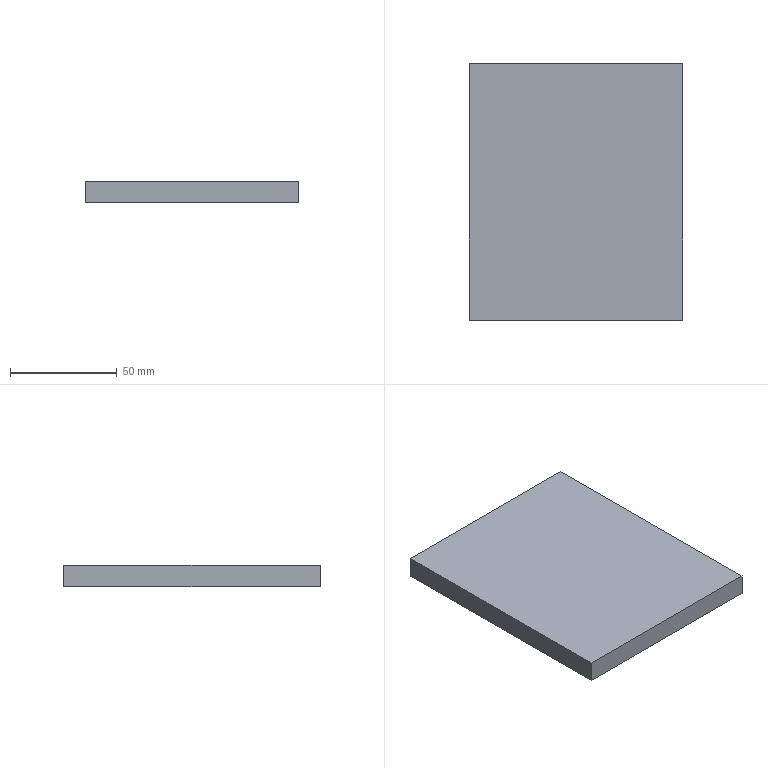Part | SolidWorks | features ICE 3, Extrusion 1 | 1 solid | 6 faces | box 100 x 120 x 10 mm | volume 120000 mm3 | plane 6
STEP:
#1=CARTESIAN_POINT('',(50.,100.,10.));
#2=VERTEX_POINT('',#1);
#3=CARTESIAN_POINT('',(50.,100.,0.));
#4=VERTEX_POINT('',#3);
#5=CARTESIAN_POINT('',(50.,100.,10.));
#6=DIRECTION('',(0.,0.,-1.));
#7=VECTOR('',#6,1000.);
#8=LINE('',#5,#7);
#9=EDGE_CURVE('',#2,#4,#8,.T.);
#10=ORIENTED_EDGE('',*,*,#9,.F.);
#11=CARTESIAN_POINT('',(50.,-20.,10.));
#12=VERTEX_POINT('',#11);
#13=CARTESIAN_POINT('',(50.,150.,10.));
#14=DIRECTION('',(0.,1.,0.));
#15=VECTOR('',#14,1000.);
#16=LINE('',#13,#15);
#17=EDGE_CURVE('',#12,#2,#16,.T.);
#18=ORIENTED_EDGE('',*,*,#17,.F.);
#19=CARTESIAN_POINT('',(50.,-20.,0.));
#20=VERTEX_POINT('',#19);
#21=CARTESIAN_POINT('',(50.,-20.,0.));
#22=DIRECTION('',(0.,0.,1.));
#23=VECTOR('',#22,1000.);
#24=LINE('',#21,#23);
#25=EDGE_CURVE('',#20,#12,#24,.T.);
#26=ORIENTED_EDGE('',*,*,#25,.F.);
#27=CARTESIAN_POINT('',(50.,150.,0.));
#28=DIRECTION('',(0.,1.,0.));
#29=VECTOR('',#28,1000.);
#30=LINE('',#27,#29);
#31=EDGE_CURVE('',#20,#4,#30,.T.);
#32=ORIENTED_EDGE('',*,*,#31,.T.);
#33=EDGE_LOOP('',(#10,#18,#26,#32));
#34=FACE_OUTER_BOUND('',#33,.T.);
#35=CARTESIAN_POINT('',(50.,150.,10.));
#36=DIRECTION('',(-1.,0.,0.));
#37=DIRECTION('',(0.,0.,1.));
#38=AXIS2_PLACEMENT_3D('',#35,#36,#37);
#39=PLANE('',#38);
#40=ADVANCED_FACE('',(#34),#39,.F.);
#41=CARTESIAN_POINT('',(-50.,100.,10.));
#42=VERTEX_POINT('',#41);
#43=CARTESIAN_POINT('',(0.,100.,10.));
#44=DIRECTION('',(1.,0.,0.));
#45=VECTOR('',#44,1000.);
#46=LINE('',#43,#45);
#47=EDGE_CURVE('',#42,#2,#46,.T.);
#48=ORIENTED_EDGE('',*,*,#47,.F.);
#49=CARTESIAN_POINT('',(-50.,-20.,10.));
#50=VERTEX_POINT('',#49);
#51=CARTESIAN_POINT('',(-50.,0.,10.));
#52=DIRECTION('',(0.,1.,0.));
#53=VECTOR('',#52,1000.);
#54=LINE('',#51,#53);
#55=EDGE_CURVE('',#50,#42,#54,.T.);
#56=ORIENTED_EDGE('',*,*,#55,.F.);
#57=CARTESIAN_POINT('',(50.,-20.,10.));
#58=DIRECTION('',(-1.,0.,0.));
#59=VECTOR('',#58,1000.);
#60=LINE('',#57,#59);
#61=EDGE_CURVE('',#12,#50,#60,.T.);
#62=ORIENTED_EDGE('',*,*,#61,.F.);
#63=ORIENTED_EDGE('',*,*,#17,.T.);
#64=EDGE_LOOP('',(#48,#56,#62,#63));
#65=FACE_OUTER_BOUND('',#64,.T.);
#66=CARTESIAN_POINT('',(0.,0.,10.));
#67=DIRECTION('',(0.,0.,-1.));
#68=DIRECTION('',(-1.,0.,0.));
#69=AXIS2_PLACEMENT_3D('',#66,#67,#68);
#70=PLANE('',#69);
#71=ADVANCED_FACE('',(#65),#70,.F.);
#72=ORIENTED_EDGE('',*,*,#31,.F.);
#73=CARTESIAN_POINT('',(-50.,-20.,0.));
#74=VERTEX_POINT('',#73);
#75=CARTESIAN_POINT('',(-50.,-20.,0.));
#76=DIRECTION('',(1.,0.,0.));
#77=VECTOR('',#76,1000.);
#78=LINE('',#75,#77);
#79=EDGE_CURVE('',#74,#20,#78,.T.);
#80=ORIENTED_EDGE('',*,*,#79,.F.);
#81=CARTESIAN_POINT('',(-50.,100.,0.));
#82=VERTEX_POINT('',#81);
#83=CARTESIAN_POINT('',(-50.,100.,0.));
#84=DIRECTION('',(0.,-1.,0.));
#85=VECTOR('',#84,1000.);
#86=LINE('',#83,#85);
#87=EDGE_CURVE('',#82,#74,#86,.T.);
#88=ORIENTED_EDGE('',*,*,#87,.F.);
#89=CARTESIAN_POINT('',(0.,100.,0.));
#90=DIRECTION('',(1.,0.,0.));
#91=VECTOR('',#90,1000.);
#92=LINE('',#89,#91);
#93=EDGE_CURVE('',#82,#4,#92,.T.);
#94=ORIENTED_EDGE('',*,*,#93,.T.);
#95=EDGE_LOOP('',(#72,#80,#88,#94));
#96=FACE_OUTER_BOUND('',#95,.T.);
#97=CARTESIAN_POINT('',(0.,0.,0.));
#98=DIRECTION('',(0.,0.,-1.));
#99=DIRECTION('',(-1.,0.,0.));
#100=AXIS2_PLACEMENT_3D('',#97,#98,#99);
#101=PLANE('',#100);
#102=ADVANCED_FACE('',(#96),#101,.T.);
#103=ORIENTED_EDGE('',*,*,#47,.T.);
#104=ORIENTED_EDGE('',*,*,#9,.T.);
#105=ORIENTED_EDGE('',*,*,#93,.F.);
#106=CARTESIAN_POINT('',(-50.,100.,10.));
#107=DIRECTION('',(0.,0.,-1.));
#108=VECTOR('',#107,1000.);
#109=LINE('',#106,#108);
#110=EDGE_CURVE('',#42,#82,#109,.T.);
#111=ORIENTED_EDGE('',*,*,#110,.F.);
#112=EDGE_LOOP('',(#103,#104,#105,#111));
#113=FACE_OUTER_BOUND('',#112,.T.);
#114=CARTESIAN_POINT('',(0.,100.,0.));
#115=DIRECTION('',(0.,1.,0.));
#116=DIRECTION('',(0.,0.,1.));
#117=AXIS2_PLACEMENT_3D('',#114,#115,#116);
#118=PLANE('',#117);
#119=ADVANCED_FACE('',(#113),#118,.T.);
#120=ORIENTED_EDGE('',*,*,#55,.T.);
#121=ORIENTED_EDGE('',*,*,#110,.T.);
#122=ORIENTED_EDGE('',*,*,#87,.T.);
#123=CARTESIAN_POINT('',(-50.,-20.,10.));
#124=DIRECTION('',(0.,0.,-1.));
#125=VECTOR('',#124,1000.);
#126=LINE('',#123,#125);
#127=EDGE_CURVE('',#50,#74,#126,.T.);
#128=ORIENTED_EDGE('',*,*,#127,.F.);
#129=EDGE_LOOP('',(#120,#121,#122,#128));
#130=FACE_OUTER_BOUND('',#129,.T.);
#131=CARTESIAN_POINT('',(-50.,0.,0.));
#132=DIRECTION('',(-1.,0.,0.));
#133=DIRECTION('',(0.,0.,1.));
#134=AXIS2_PLACEMENT_3D('',#131,#132,#133);
#135=PLANE('',#134);
#136=ADVANCED_FACE('',(#130),#135,.T.);
#137=ORIENTED_EDGE('',*,*,#127,.T.);
#138=ORIENTED_EDGE('',*,*,#79,.T.);
#139=ORIENTED_EDGE('',*,*,#25,.T.);
#140=ORIENTED_EDGE('',*,*,#61,.T.);
#141=EDGE_LOOP('',(#137,#138,#139,#140));
#142=FACE_OUTER_BOUND('',#141,.T.);
#143=CARTESIAN_POINT('',(0.,-20.,0.));
#144=DIRECTION('',(0.,-1.,0.));
#145=DIRECTION('',(0.,0.,-1.));
#146=AXIS2_PLACEMENT_3D('',#143,#144,#145);
#147=PLANE('',#146);
#148=ADVANCED_FACE('',(#142),#147,.T.);
#149=CLOSED_SHELL('',(#40,#71,#102,#119,#136,#148));
#150=MANIFOLD_SOLID_BREP('',#149);
#151=CARTESIAN_POINT('',(0.,0.,0.));
#152=DIRECTION('',(0.,0.,1.));
#153=DIRECTION('',(1.,0.,0.));
#154=AXIS2_PLACEMENT_3D('',#151,#152,#153);
#155=(LENGTH_UNIT()NAMED_UNIT(*)SI_UNIT(.MILLI.,.METRE.));
#156=UNCERTAINTY_MEASURE_WITH_UNIT(LENGTH_MEASURE(0.00001),#155,'','');
#157=(NAMED_UNIT(*)PLANE_ANGLE_UNIT()SI_UNIT($,.RADIAN.));
#158=(NAMED_UNIT(*)SI_UNIT($,.STERADIAN.)SOLID_ANGLE_UNIT());
#159=(GEOMETRIC_REPRESENTATION_CONTEXT(3)GLOBAL_UNCERTAINTY_ASSIGNED_CONTEXT((#156))GLOBAL_UNIT_ASSIGNED_CONTEXT((#155,#157,#158))REPRESENTATION_CONTEXT('',''));
#160=ADVANCED_BREP_SHAPE_REPRESENTATION('',(#150,#154),#159);